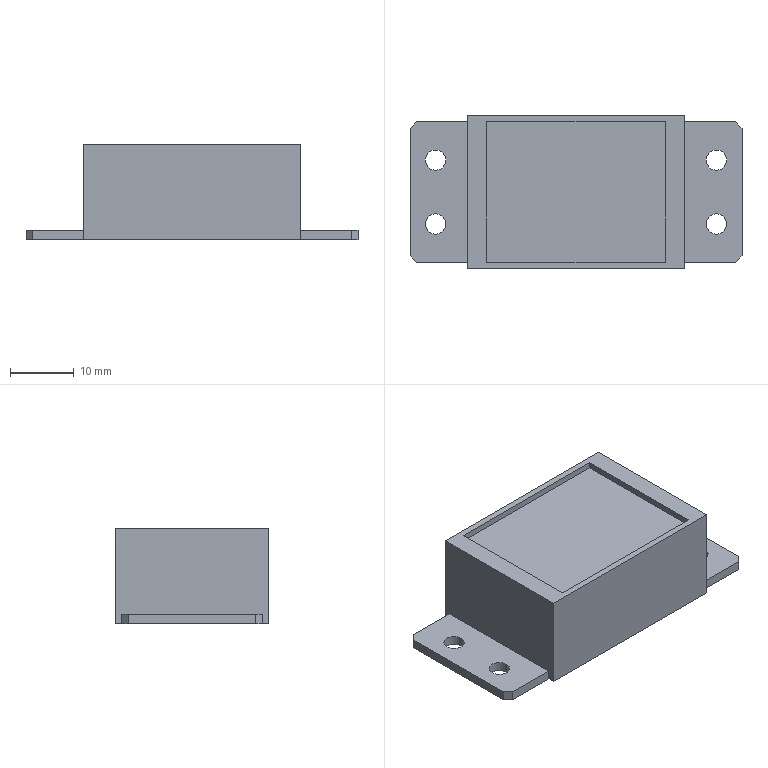Part | STEP file | V-light-BGS3-D20-R-W | 1 solid | 31 faces | box 52 x 24 x 15 mm | volume 12167 mm3 | plane 23 | cylinder 8 | commonest cylinder face diameters 3.2 x8
STEP:
#1=CARTESIAN_POINT('',(20.4,5.,0.));
#2=VERTEX_POINT('',#1);
#3=CARTESIAN_POINT('',(23.6,5.,0.));
#4=VERTEX_POINT('',#3);
#5=CARTESIAN_POINT('',(22.,5.,0.));
#6=DIRECTION('',(0.,0.,1.));
#7=DIRECTION('',(-1.,0.,0.));
#8=AXIS2_PLACEMENT_3D('',#5,#6,#7);
#9=CIRCLE('',#8,1.6);
#10=EDGE_CURVE('',#2,#4,#9,.T.);
#11=ORIENTED_EDGE('',*,*,#10,.F.);
#12=CARTESIAN_POINT('',(20.4,5.,1.5));
#13=VERTEX_POINT('',#12);
#14=CARTESIAN_POINT('',(20.4,5.,0.));
#15=DIRECTION('',(0.,0.,1.));
#16=VECTOR('',#15,1000.);
#17=LINE('',#14,#16);
#18=EDGE_CURVE('',#2,#13,#17,.T.);
#19=ORIENTED_EDGE('',*,*,#18,.T.);
#20=CARTESIAN_POINT('',(23.6,5.,1.5));
#21=VERTEX_POINT('',#20);
#22=CARTESIAN_POINT('',(22.,5.,1.5));
#23=DIRECTION('',(0.,0.,1.));
#24=DIRECTION('',(-1.,0.,0.));
#25=AXIS2_PLACEMENT_3D('',#22,#23,#24);
#26=CIRCLE('',#25,1.6);
#27=EDGE_CURVE('',#13,#21,#26,.T.);
#28=ORIENTED_EDGE('',*,*,#27,.T.);
#29=CARTESIAN_POINT('',(23.6,5.,0.));
#30=DIRECTION('',(0.,0.,1.));
#31=VECTOR('',#30,1000.);
#32=LINE('',#29,#31);
#33=EDGE_CURVE('',#4,#21,#32,.T.);
#34=ORIENTED_EDGE('',*,*,#33,.F.);
#35=EDGE_LOOP('',(#11,#19,#28,#34));
#36=FACE_OUTER_BOUND('',#35,.T.);
#37=CARTESIAN_POINT('',(22.,5.,0.));
#38=DIRECTION('',(0.,0.,1.));
#39=DIRECTION('',(1.,0.,0.));
#40=AXIS2_PLACEMENT_3D('',#37,#38,#39);
#41=CYLINDRICAL_SURFACE('',#40,1.6);
#42=ADVANCED_FACE('',(#36),#41,.F.);
#43=CARTESIAN_POINT('',(20.4,-5.,0.));
#44=VERTEX_POINT('',#43);
#45=CARTESIAN_POINT('',(23.6,-5.,0.));
#46=VERTEX_POINT('',#45);
#47=CARTESIAN_POINT('',(22.,-5.,0.));
#48=DIRECTION('',(0.,0.,1.));
#49=DIRECTION('',(1.,0.,0.));
#50=AXIS2_PLACEMENT_3D('',#47,#48,#49);
#51=CIRCLE('',#50,1.6);
#52=EDGE_CURVE('',#44,#46,#51,.T.);
#53=ORIENTED_EDGE('',*,*,#52,.F.);
#54=CARTESIAN_POINT('',(20.4,-5.,1.5));
#55=VERTEX_POINT('',#54);
#56=CARTESIAN_POINT('',(20.4,-5.,0.));
#57=DIRECTION('',(0.,0.,1.));
#58=VECTOR('',#57,1000.);
#59=LINE('',#56,#58);
#60=EDGE_CURVE('',#44,#55,#59,.T.);
#61=ORIENTED_EDGE('',*,*,#60,.T.);
#62=CARTESIAN_POINT('',(23.6,-5.,1.5));
#63=VERTEX_POINT('',#62);
#64=CARTESIAN_POINT('',(22.,-5.,1.5));
#65=DIRECTION('',(0.,0.,1.));
#66=DIRECTION('',(1.,0.,0.));
#67=AXIS2_PLACEMENT_3D('',#64,#65,#66);
#68=CIRCLE('',#67,1.6);
#69=EDGE_CURVE('',#55,#63,#68,.T.);
#70=ORIENTED_EDGE('',*,*,#69,.T.);
#71=CARTESIAN_POINT('',(23.6,-5.,0.));
#72=DIRECTION('',(0.,0.,1.));
#73=VECTOR('',#72,1000.);
#74=LINE('',#71,#73);
#75=EDGE_CURVE('',#46,#63,#74,.T.);
#76=ORIENTED_EDGE('',*,*,#75,.F.);
#77=EDGE_LOOP('',(#53,#61,#70,#76));
#78=FACE_OUTER_BOUND('',#77,.T.);
#79=CARTESIAN_POINT('',(22.,-5.,0.));
#80=DIRECTION('',(0.,0.,1.));
#81=DIRECTION('',(1.,0.,0.));
#82=AXIS2_PLACEMENT_3D('',#79,#80,#81);
#83=CYLINDRICAL_SURFACE('',#82,1.6);
#84=ADVANCED_FACE('',(#78),#83,.F.);
#85=CARTESIAN_POINT('',(-23.6,-5.,0.));
#86=VERTEX_POINT('',#85);
#87=CARTESIAN_POINT('',(-20.4,-5.,0.));
#88=VERTEX_POINT('',#87);
#89=CARTESIAN_POINT('',(-22.,-5.,0.));
#90=DIRECTION('',(0.,0.,1.));
#91=DIRECTION('',(-1.,0.,0.));
#92=AXIS2_PLACEMENT_3D('',#89,#90,#91);
#93=CIRCLE('',#92,1.6);
#94=EDGE_CURVE('',#86,#88,#93,.T.);
#95=ORIENTED_EDGE('',*,*,#94,.F.);
#96=CARTESIAN_POINT('',(-23.6,-5.,1.5));
#97=VERTEX_POINT('',#96);
#98=CARTESIAN_POINT('',(-23.6,-5.,0.));
#99=DIRECTION('',(0.,0.,1.));
#100=VECTOR('',#99,1000.);
#101=LINE('',#98,#100);
#102=EDGE_CURVE('',#86,#97,#101,.T.);
#103=ORIENTED_EDGE('',*,*,#102,.T.);
#104=CARTESIAN_POINT('',(-20.4,-5.,1.5));
#105=VERTEX_POINT('',#104);
#106=CARTESIAN_POINT('',(-22.,-5.,1.5));
#107=DIRECTION('',(0.,0.,1.));
#108=DIRECTION('',(-1.,0.,0.));
#109=AXIS2_PLACEMENT_3D('',#106,#107,#108);
#110=CIRCLE('',#109,1.6);
#111=EDGE_CURVE('',#97,#105,#110,.T.);
#112=ORIENTED_EDGE('',*,*,#111,.T.);
#113=CARTESIAN_POINT('',(-20.4,-5.,0.));
#114=DIRECTION('',(0.,0.,1.));
#115=VECTOR('',#114,1000.);
#116=LINE('',#113,#115);
#117=EDGE_CURVE('',#88,#105,#116,.T.);
#118=ORIENTED_EDGE('',*,*,#117,.F.);
#119=EDGE_LOOP('',(#95,#103,#112,#118));
#120=FACE_OUTER_BOUND('',#119,.T.);
#121=CARTESIAN_POINT('',(-22.,-5.,0.));
#122=DIRECTION('',(0.,0.,1.));
#123=DIRECTION('',(1.,0.,0.));
#124=AXIS2_PLACEMENT_3D('',#121,#122,#123);
#125=CYLINDRICAL_SURFACE('',#124,1.6);
#126=ADVANCED_FACE('',(#120),#125,.F.);
#127=CARTESIAN_POINT('',(-23.6,5.,0.));
#128=VERTEX_POINT('',#127);
#129=CARTESIAN_POINT('',(-20.4,5.,0.));
#130=VERTEX_POINT('',#129);
#131=CARTESIAN_POINT('',(-22.,5.,0.));
#132=DIRECTION('',(0.,0.,1.));
#133=DIRECTION('',(1.,0.,0.));
#134=AXIS2_PLACEMENT_3D('',#131,#132,#133);
#135=CIRCLE('',#134,1.6);
#136=EDGE_CURVE('',#128,#130,#135,.T.);
#137=ORIENTED_EDGE('',*,*,#136,.F.);
#138=CARTESIAN_POINT('',(-23.6,5.,1.5));
#139=VERTEX_POINT('',#138);
#140=CARTESIAN_POINT('',(-23.6,5.,0.));
#141=DIRECTION('',(0.,0.,1.));
#142=VECTOR('',#141,1000.);
#143=LINE('',#140,#142);
#144=EDGE_CURVE('',#128,#139,#143,.T.);
#145=ORIENTED_EDGE('',*,*,#144,.T.);
#146=CARTESIAN_POINT('',(-20.4,5.,1.5));
#147=VERTEX_POINT('',#146);
#148=CARTESIAN_POINT('',(-22.,5.,1.5));
#149=DIRECTION('',(0.,0.,1.));
#150=DIRECTION('',(1.,0.,0.));
#151=AXIS2_PLACEMENT_3D('',#148,#149,#150);
#152=CIRCLE('',#151,1.6);
#153=EDGE_CURVE('',#139,#147,#152,.T.);
#154=ORIENTED_EDGE('',*,*,#153,.T.);
#155=CARTESIAN_POINT('',(-20.4,5.,0.));
#156=DIRECTION('',(0.,0.,1.));
#157=VECTOR('',#156,1000.);
#158=LINE('',#155,#157);
#159=EDGE_CURVE('',#130,#147,#158,.T.);
#160=ORIENTED_EDGE('',*,*,#159,.F.);
#161=EDGE_LOOP('',(#137,#145,#154,#160));
#162=FACE_OUTER_BOUND('',#161,.T.);
#163=CARTESIAN_POINT('',(-22.,5.,0.));
#164=DIRECTION('',(0.,0.,1.));
#165=DIRECTION('',(1.,0.,0.));
#166=AXIS2_PLACEMENT_3D('',#163,#164,#165);
#167=CYLINDRICAL_SURFACE('',#166,1.6);
#168=ADVANCED_FACE('',(#162),#167,.F.);
#169=CARTESIAN_POINT('',(25.,-11.,1.5));
#170=VERTEX_POINT('',#169);
#171=CARTESIAN_POINT('',(17.,-11.,1.5));
#172=VERTEX_POINT('',#171);
#173=CARTESIAN_POINT('',(26.,-11.,1.5));
#174=DIRECTION('',(-1.,0.,0.));
#175=VECTOR('',#174,1000.);
#176=LINE('',#173,#175);
#177=EDGE_CURVE('',#170,#172,#176,.T.);
#178=ORIENTED_EDGE('',*,*,#177,.F.);
#179=CARTESIAN_POINT('',(26.,-10.,1.5));
#180=VERTEX_POINT('',#179);
#181=CARTESIAN_POINT('',(25.,-11.,1.5));
#182=DIRECTION('',(0.7071,0.7071,0.));
#183=VECTOR('',#182,1000.);
#184=LINE('',#181,#183);
#185=EDGE_CURVE('',#170,#180,#184,.T.);
#186=ORIENTED_EDGE('',*,*,#185,.T.);
#187=CARTESIAN_POINT('',(26.,10.,1.5));
#188=VERTEX_POINT('',#187);
#189=CARTESIAN_POINT('',(26.,12.,1.5));
#190=DIRECTION('',(0.,1.,0.));
#191=VECTOR('',#190,1000.);
#192=LINE('',#189,#191);
#193=EDGE_CURVE('',#180,#188,#192,.T.);
#194=ORIENTED_EDGE('',*,*,#193,.T.);
#195=CARTESIAN_POINT('',(25.,11.,1.5));
#196=VERTEX_POINT('',#195);
#197=CARTESIAN_POINT('',(37.,-1.,1.5));
#198=DIRECTION('',(-0.7071,0.7071,0.));
#199=VECTOR('',#198,1000.);
#200=LINE('',#197,#199);
#201=EDGE_CURVE('',#188,#196,#200,.T.);
#202=ORIENTED_EDGE('',*,*,#201,.T.);
#203=CARTESIAN_POINT('',(17.,11.,1.5));
#204=VERTEX_POINT('',#203);
#205=CARTESIAN_POINT('',(17.,11.,1.5));
#206=DIRECTION('',(1.,0.,0.));
#207=VECTOR('',#206,1000.);
#208=LINE('',#205,#207);
#209=EDGE_CURVE('',#204,#196,#208,.T.);
#210=ORIENTED_EDGE('',*,*,#209,.F.);
#211=CARTESIAN_POINT('',(17.,-12.,1.5));
#212=DIRECTION('',(0.,1.,0.));
#213=VECTOR('',#212,1000.);
#214=LINE('',#211,#213);
#215=EDGE_CURVE('',#172,#204,#214,.T.);
#216=ORIENTED_EDGE('',*,*,#215,.F.);
#217=EDGE_LOOP('',(#178,#186,#194,#202,#210,#216));
#218=FACE_OUTER_BOUND('',#217,.T.);
#219=CARTESIAN_POINT('',(22.,-5.,1.5));
#220=DIRECTION('',(0.,0.,1.));
#221=DIRECTION('',(1.,0.,0.));
#222=AXIS2_PLACEMENT_3D('',#219,#220,#221);
#223=CIRCLE('',#222,1.6);
#224=EDGE_CURVE('',#63,#55,#223,.T.);
#225=ORIENTED_EDGE('',*,*,#224,.F.);
#226=ORIENTED_EDGE('',*,*,#69,.F.);
#227=EDGE_LOOP('',(#225,#226));
#228=FACE_BOUND('',#227,.T.);
#229=CARTESIAN_POINT('',(22.,5.,1.5));
#230=DIRECTION('',(0.,0.,1.));
#231=DIRECTION('',(-1.,0.,0.));
#232=AXIS2_PLACEMENT_3D('',#229,#230,#231);
#233=CIRCLE('',#232,1.6);
#234=EDGE_CURVE('',#21,#13,#233,.T.);
#235=ORIENTED_EDGE('',*,*,#234,.F.);
#236=ORIENTED_EDGE('',*,*,#27,.F.);
#237=EDGE_LOOP('',(#235,#236));
#238=FACE_BOUND('',#237,.T.);
#239=CARTESIAN_POINT('',(26.,-12.,1.5));
#240=DIRECTION('',(0.,0.,1.));
#241=DIRECTION('',(1.,0.,0.));
#242=AXIS2_PLACEMENT_3D('',#239,#240,#241);
#243=PLANE('',#242);
#244=ADVANCED_FACE('',(#218,#228,#238),#243,.T.);
#245=ORIENTED_EDGE('',*,*,#193,.F.);
#246=CARTESIAN_POINT('',(26.,-10.,0.));
#247=VERTEX_POINT('',#246);
#248=CARTESIAN_POINT('',(26.,-10.,1.5));
#249=DIRECTION('',(0.,0.,-1.));
#250=VECTOR('',#249,1000.);
#251=LINE('',#248,#250);
#252=EDGE_CURVE('',#180,#247,#251,.T.);
#253=ORIENTED_EDGE('',*,*,#252,.T.);
#254=CARTESIAN_POINT('',(26.,10.,0.));
#255=VERTEX_POINT('',#254);
#256=CARTESIAN_POINT('',(26.,12.,0.));
#257=DIRECTION('',(0.,1.,0.));
#258=VECTOR('',#257,1000.);
#259=LINE('',#256,#258);
#260=EDGE_CURVE('',#247,#255,#259,.T.);
#261=ORIENTED_EDGE('',*,*,#260,.T.);
#262=CARTESIAN_POINT('',(26.,10.,1.5));
#263=DIRECTION('',(0.,0.,1.));
#264=VECTOR('',#263,1000.);
#265=LINE('',#262,#264);
#266=EDGE_CURVE('',#255,#188,#265,.T.);
#267=ORIENTED_EDGE('',*,*,#266,.T.);
#268=EDGE_LOOP('',(#245,#253,#261,#267));
#269=FACE_OUTER_BOUND('',#268,.T.);
#270=CARTESIAN_POINT('',(26.,12.,1.5));
#271=DIRECTION('',(-1.,0.,0.));
#272=DIRECTION('',(0.,-1.,0.));
#273=AXIS2_PLACEMENT_3D('',#270,#271,#272);
#274=PLANE('',#273);
#275=ADVANCED_FACE('',(#269),#274,.F.);
#276=CARTESIAN_POINT('',(17.,12.,0.));
#277=VERTEX_POINT('',#276);
#278=CARTESIAN_POINT('',(-17.,12.,0.));
#279=VERTEX_POINT('',#278);
#280=CARTESIAN_POINT('',(-26.,12.,0.));
#281=DIRECTION('',(-1.,0.,0.));
#282=VECTOR('',#281,1000.);
#283=LINE('',#280,#282);
#284=EDGE_CURVE('',#277,#279,#283,.T.);
#285=ORIENTED_EDGE('',*,*,#284,.T.);
#286=CARTESIAN_POINT('',(-17.,12.,15.));
#287=VERTEX_POINT('',#286);
#288=CARTESIAN_POINT('',(-17.,12.,15.));
#289=DIRECTION('',(0.,0.,-1.));
#290=VECTOR('',#289,1000.);
#291=LINE('',#288,#290);
#292=EDGE_CURVE('',#287,#279,#291,.T.);
#293=ORIENTED_EDGE('',*,*,#292,.F.);
#294=CARTESIAN_POINT('',(17.,12.,15.));
#295=VERTEX_POINT('',#294);
#296=CARTESIAN_POINT('',(-17.,12.,15.));
#297=DIRECTION('',(-1.,0.,0.));
#298=VECTOR('',#297,1000.);
#299=LINE('',#296,#298);
#300=EDGE_CURVE('',#295,#287,#299,.T.);
#301=ORIENTED_EDGE('',*,*,#300,.F.);
#302=CARTESIAN_POINT('',(17.,12.,15.));
#303=DIRECTION('',(0.,0.,-1.));
#304=VECTOR('',#303,1000.);
#305=LINE('',#302,#304);
#306=EDGE_CURVE('',#295,#277,#305,.T.);
#307=ORIENTED_EDGE('',*,*,#306,.T.);
#308=EDGE_LOOP('',(#285,#293,#301,#307));
#309=FACE_OUTER_BOUND('',#308,.T.);
#310=CARTESIAN_POINT('',(-26.,12.,1.5));
#311=DIRECTION('',(0.,-1.,0.));
#312=DIRECTION('',(0.,0.,-1.));
#313=AXIS2_PLACEMENT_3D('',#310,#311,#312);
#314=PLANE('',#313);
#315=ADVANCED_FACE('',(#309),#314,.F.);
#316=CARTESIAN_POINT('',(-26.,10.,0.));
#317=VERTEX_POINT('',#316);
#318=CARTESIAN_POINT('',(-26.,-10.,0.));
#319=VERTEX_POINT('',#318);
#320=CARTESIAN_POINT('',(-26.,12.,0.));
#321=DIRECTION('',(0.,-1.,0.));
#322=VECTOR('',#321,1000.);
#323=LINE('',#320,#322);
#324=EDGE_CURVE('',#317,#319,#323,.T.);
#325=ORIENTED_EDGE('',*,*,#324,.T.);
#326=CARTESIAN_POINT('',(-26.,-10.,1.5));
#327=VERTEX_POINT('',#326);
#328=CARTESIAN_POINT('',(-26.,-10.,1.5));
#329=DIRECTION('',(0.,0.,1.));
#330=VECTOR('',#329,1000.);
#331=LINE('',#328,#330);
#332=EDGE_CURVE('',#319,#327,#331,.T.);
#333=ORIENTED_EDGE('',*,*,#332,.T.);
#334=CARTESIAN_POINT('',(-26.,10.,1.5));
#335=VERTEX_POINT('',#334);
#336=CARTESIAN_POINT('',(-26.,12.,1.5));
#337=DIRECTION('',(0.,-1.,0.));
#338=VECTOR('',#337,1000.);
#339=LINE('',#336,#338);
#340=EDGE_CURVE('',#335,#327,#339,.T.);
#341=ORIENTED_EDGE('',*,*,#340,.F.);
#342=CARTESIAN_POINT('',(-26.,10.,1.5));
#343=DIRECTION('',(0.,0.,-1.));
#344=VECTOR('',#343,1000.);
#345=LINE('',#342,#344);
#346=EDGE_CURVE('',#335,#317,#345,.T.);
#347=ORIENTED_EDGE('',*,*,#346,.T.);
#348=EDGE_LOOP('',(#325,#333,#341,#347));
#349=FACE_OUTER_BOUND('',#348,.T.);
#350=CARTESIAN_POINT('',(-26.,12.,1.5));
#351=DIRECTION('',(1.,0.,0.));
#352=DIRECTION('',(0.,1.,0.));
#353=AXIS2_PLACEMENT_3D('',#350,#351,#352);
#354=PLANE('',#353);
#355=ADVANCED_FACE('',(#349),#354,.F.);
#356=CARTESIAN_POINT('',(-17.,-12.,15.));
#357=VERTEX_POINT('',#356);
#358=CARTESIAN_POINT('',(-17.,-12.,0.));
#359=VERTEX_POINT('',#358);
#360=CARTESIAN_POINT('',(-17.,-12.,15.));
#361=DIRECTION('',(0.,0.,-1.));
#362=VECTOR('',#361,1000.);
#363=LINE('',#360,#362);
#364=EDGE_CURVE('',#357,#359,#363,.T.);
#365=ORIENTED_EDGE('',*,*,#364,.T.);
#366=CARTESIAN_POINT('',(17.,-12.,0.));
#367=VERTEX_POINT('',#366);
#368=CARTESIAN_POINT('',(-26.,-12.,0.));
#369=DIRECTION('',(1.,0.,0.));
#370=VECTOR('',#369,1000.);
#371=LINE('',#368,#370);
#372=EDGE_CURVE('',#359,#367,#371,.T.);
#373=ORIENTED_EDGE('',*,*,#372,.T.);
#374=CARTESIAN_POINT('',(17.,-12.,15.));
#375=VERTEX_POINT('',#374);
#376=CARTESIAN_POINT('',(17.,-12.,15.));
#377=DIRECTION('',(0.,0.,-1.));
#378=VECTOR('',#377,1000.);
#379=LINE('',#376,#378);
#380=EDGE_CURVE('',#375,#367,#379,.T.);
#381=ORIENTED_EDGE('',*,*,#380,.F.);
#382=CARTESIAN_POINT('',(-17.,-12.,15.));
#383=DIRECTION('',(1.,0.,0.));
#384=VECTOR('',#383,1000.);
#385=LINE('',#382,#384);
#386=EDGE_CURVE('',#357,#375,#385,.T.);
#387=ORIENTED_EDGE('',*,*,#386,.F.);
#388=EDGE_LOOP('',(#365,#373,#381,#387));
#389=FACE_OUTER_BOUND('',#388,.T.);
#390=CARTESIAN_POINT('',(-26.,-12.,1.5));
#391=DIRECTION('',(0.,1.,0.));
#392=DIRECTION('',(0.,0.,1.));
#393=AXIS2_PLACEMENT_3D('',#390,#391,#392);
#394=PLANE('',#393);
#395=ADVANCED_FACE('',(#389),#394,.F.);
#396=ORIENTED_EDGE('',*,*,#340,.T.);
#397=CARTESIAN_POINT('',(-25.,-11.,1.5));
#398=VERTEX_POINT('',#397);
#399=CARTESIAN_POINT('',(1.,-37.,1.5));
#400=DIRECTION('',(0.7071,-0.7071,0.));
#401=VECTOR('',#400,1000.);
#402=LINE('',#399,#401);
#403=EDGE_CURVE('',#327,#398,#402,.T.);
#404=ORIENTED_EDGE('',*,*,#403,.T.);
#405=CARTESIAN_POINT('',(-17.,-11.,1.5));
#406=VERTEX_POINT('',#405);
#407=CARTESIAN_POINT('',(-26.,-11.,1.5));
#408=DIRECTION('',(-1.,0.,0.));
#409=VECTOR('',#408,1000.);
#410=LINE('',#407,#409);
#411=EDGE_CURVE('',#406,#398,#410,.T.);
#412=ORIENTED_EDGE('',*,*,#411,.F.);
#413=CARTESIAN_POINT('',(-17.,11.,1.5));
#414=VERTEX_POINT('',#413);
#415=CARTESIAN_POINT('',(-17.,-12.,1.5));
#416=DIRECTION('',(0.,-1.,0.));
#417=VECTOR('',#416,1000.);
#418=LINE('',#415,#417);
#419=EDGE_CURVE('',#414,#406,#418,.T.);
#420=ORIENTED_EDGE('',*,*,#419,.F.);
#421=CARTESIAN_POINT('',(-25.,11.,1.5));
#422=VERTEX_POINT('',#421);
#423=CARTESIAN_POINT('',(-17.,11.,1.5));
#424=DIRECTION('',(1.,0.,0.));
#425=VECTOR('',#424,1000.);
#426=LINE('',#423,#425);
#427=EDGE_CURVE('',#422,#414,#426,.T.);
#428=ORIENTED_EDGE('',*,*,#427,.F.);
#429=CARTESIAN_POINT('',(-11.,25.,1.5));
#430=DIRECTION('',(-0.7071,-0.7071,0.));
#431=VECTOR('',#430,1000.);
#432=LINE('',#429,#431);
#433=EDGE_CURVE('',#422,#335,#432,.T.);
#434=ORIENTED_EDGE('',*,*,#433,.T.);
#435=EDGE_LOOP('',(#396,#404,#412,#420,#428,#434));
#436=FACE_OUTER_BOUND('',#435,.T.);
#437=CARTESIAN_POINT('',(-22.,-5.,1.5));
#438=DIRECTION('',(0.,0.,1.));
#439=DIRECTION('',(-1.,0.,0.));
#440=AXIS2_PLACEMENT_3D('',#437,#438,#439);
#441=CIRCLE('',#440,1.6);
#442=EDGE_CURVE('',#105,#97,#441,.T.);
#443=ORIENTED_EDGE('',*,*,#442,.F.);
#444=ORIENTED_EDGE('',*,*,#111,.F.);
#445=EDGE_LOOP('',(#443,#444));
#446=FACE_BOUND('',#445,.T.);
#447=CARTESIAN_POINT('',(-22.,5.,1.5));
#448=DIRECTION('',(0.,0.,1.));
#449=DIRECTION('',(1.,0.,0.));
#450=AXIS2_PLACEMENT_3D('',#447,#448,#449);
#451=CIRCLE('',#450,1.6);
#452=EDGE_CURVE('',#147,#139,#451,.T.);
#453=ORIENTED_EDGE('',*,*,#452,.F.);
#454=ORIENTED_EDGE('',*,*,#153,.F.);
#455=EDGE_LOOP('',(#453,#454));
#456=FACE_BOUND('',#455,.T.);
#457=CARTESIAN_POINT('',(26.,-12.,1.5));
#458=DIRECTION('',(0.,0.,1.));
#459=DIRECTION('',(1.,0.,0.));
#460=AXIS2_PLACEMENT_3D('',#457,#458,#459);
#461=PLANE('',#460);
#462=ADVANCED_FACE('',(#436,#446,#456),#461,.T.);
#463=CARTESIAN_POINT('',(22.,5.,0.));
#464=DIRECTION('',(0.,0.,1.));
#465=DIRECTION('',(-1.,0.,0.));
#466=AXIS2_PLACEMENT_3D('',#463,#464,#465);
#467=CIRCLE('',#466,1.6);
#468=EDGE_CURVE('',#4,#2,#467,.T.);
#469=ORIENTED_EDGE('',*,*,#468,.T.);
#470=ORIENTED_EDGE('',*,*,#10,.T.);
#471=EDGE_LOOP('',(#469,#470));
#472=FACE_BOUND('',#471,.T.);
#473=CARTESIAN_POINT('',(22.,-5.,0.));
#474=DIRECTION('',(0.,0.,1.));
#475=DIRECTION('',(1.,0.,0.));
#476=AXIS2_PLACEMENT_3D('',#473,#474,#475);
#477=CIRCLE('',#476,1.6);
#478=EDGE_CURVE('',#46,#44,#477,.T.);
#479=ORIENTED_EDGE('',*,*,#478,.T.);
#480=ORIENTED_EDGE('',*,*,#52,.T.);
#481=EDGE_LOOP('',(#479,#480));
#482=FACE_BOUND('',#481,.T.);
#483=CARTESIAN_POINT('',(-22.,-5.,0.));
#484=DIRECTION('',(0.,0.,1.));
#485=DIRECTION('',(-1.,0.,0.));
#486=AXIS2_PLACEMENT_3D('',#483,#484,#485);
#487=CIRCLE('',#486,1.6);
#488=EDGE_CURVE('',#88,#86,#487,.T.);
#489=ORIENTED_EDGE('',*,*,#488,.T.);
#490=ORIENTED_EDGE('',*,*,#94,.T.);
#491=EDGE_LOOP('',(#489,#490));
#492=FACE_BOUND('',#491,.T.);
#493=CARTESIAN_POINT('',(-22.,5.,0.));
#494=DIRECTION('',(0.,0.,1.));
#495=DIRECTION('',(1.,0.,0.));
#496=AXIS2_PLACEMENT_3D('',#493,#494,#495);
#497=CIRCLE('',#496,1.6);
#498=EDGE_CURVE('',#130,#128,#497,.T.);
#499=ORIENTED_EDGE('',*,*,#498,.T.);
#500=ORIENTED_EDGE('',*,*,#136,.T.);
#501=EDGE_LOOP('',(#499,#500));
#502=FACE_BOUND('',#501,.T.);
#503=CARTESIAN_POINT('',(-17.,-11.,0.));
#504=VERTEX_POINT('',#503);
#505=CARTESIAN_POINT('',(-25.,-11.,0.));
#506=VERTEX_POINT('',#505);
#507=CARTESIAN_POINT('',(26.,-11.,0.));
#508=DIRECTION('',(-1.,0.,0.));
#509=VECTOR('',#508,1000.);
#510=LINE('',#507,#509);
#511=EDGE_CURVE('',#504,#506,#510,.T.);
#512=ORIENTED_EDGE('',*,*,#511,.T.);
#513=CARTESIAN_POINT('',(-26.,-10.,0.));
#514=DIRECTION('',(-0.7071,0.7071,0.));
#515=VECTOR('',#514,1000.);
#516=LINE('',#513,#515);
#517=EDGE_CURVE('',#506,#319,#516,.T.);
#518=ORIENTED_EDGE('',*,*,#517,.T.);
#519=ORIENTED_EDGE('',*,*,#324,.F.);
#520=CARTESIAN_POINT('',(-25.,11.,0.));
#521=VERTEX_POINT('',#520);
#522=CARTESIAN_POINT('',(-26.,10.,0.));
#523=DIRECTION('',(0.7071,0.7071,0.));
#524=VECTOR('',#523,1000.);
#525=LINE('',#522,#524);
#526=EDGE_CURVE('',#317,#521,#525,.T.);
#527=ORIENTED_EDGE('',*,*,#526,.T.);
#528=CARTESIAN_POINT('',(-17.,11.,0.));
#529=VERTEX_POINT('',#528);
#530=CARTESIAN_POINT('',(26.,11.,0.));
#531=DIRECTION('',(1.,0.,0.));
#532=VECTOR('',#531,1000.);
#533=LINE('',#530,#532);
#534=EDGE_CURVE('',#521,#529,#533,.T.);
#535=ORIENTED_EDGE('',*,*,#534,.T.);
#536=CARTESIAN_POINT('',(-17.,-12.,0.));
#537=DIRECTION('',(0.,1.,0.));
#538=VECTOR('',#537,1000.);
#539=LINE('',#536,#538);
#540=EDGE_CURVE('',#529,#279,#539,.T.);
#541=ORIENTED_EDGE('',*,*,#540,.T.);
#542=ORIENTED_EDGE('',*,*,#284,.F.);
#543=CARTESIAN_POINT('',(17.,11.,0.));
#544=VERTEX_POINT('',#543);
#545=CARTESIAN_POINT('',(17.,-12.,0.));
#546=DIRECTION('',(0.,-1.,0.));
#547=VECTOR('',#546,1000.);
#548=LINE('',#545,#547);
#549=EDGE_CURVE('',#277,#544,#548,.T.);
#550=ORIENTED_EDGE('',*,*,#549,.T.);
#551=CARTESIAN_POINT('',(25.,11.,0.));
#552=VERTEX_POINT('',#551);
#553=CARTESIAN_POINT('',(26.,11.,0.));
#554=DIRECTION('',(1.,0.,0.));
#555=VECTOR('',#554,1000.);
#556=LINE('',#553,#555);
#557=EDGE_CURVE('',#544,#552,#556,.T.);
#558=ORIENTED_EDGE('',*,*,#557,.T.);
#559=CARTESIAN_POINT('',(26.,10.,0.));
#560=DIRECTION('',(0.7071,-0.7071,0.));
#561=VECTOR('',#560,1000.);
#562=LINE('',#559,#561);
#563=EDGE_CURVE('',#552,#255,#562,.T.);
#564=ORIENTED_EDGE('',*,*,#563,.T.);
#565=ORIENTED_EDGE('',*,*,#260,.F.);
#566=CARTESIAN_POINT('',(25.,-11.,0.));
#567=VERTEX_POINT('',#566);
#568=CARTESIAN_POINT('',(25.,-11.,0.));
#569=DIRECTION('',(-0.7071,-0.7071,0.));
#570=VECTOR('',#569,1000.);
#571=LINE('',#568,#570);
#572=EDGE_CURVE('',#247,#567,#571,.T.);
#573=ORIENTED_EDGE('',*,*,#572,.T.);
#574=CARTESIAN_POINT('',(17.,-11.,0.));
#575=VERTEX_POINT('',#574);
#576=CARTESIAN_POINT('',(26.,-11.,0.));
#577=DIRECTION('',(-1.,0.,0.));
#578=VECTOR('',#577,1000.);
#579=LINE('',#576,#578);
#580=EDGE_CURVE('',#567,#575,#579,.T.);
#581=ORIENTED_EDGE('',*,*,#580,.T.);
#582=CARTESIAN_POINT('',(17.,-12.,0.));
#583=DIRECTION('',(0.,-1.,0.));
#584=VECTOR('',#583,1000.);
#585=LINE('',#582,#584);
#586=EDGE_CURVE('',#575,#367,#585,.T.);
#587=ORIENTED_EDGE('',*,*,#586,.T.);
#588=ORIENTED_EDGE('',*,*,#372,.F.);
#589=CARTESIAN_POINT('',(-17.,-12.,0.));
#590=DIRECTION('',(0.,1.,0.));
#591=VECTOR('',#590,1000.);
#592=LINE('',#589,#591);
#593=EDGE_CURVE('',#359,#504,#592,.T.);
#594=ORIENTED_EDGE('',*,*,#593,.T.);
#595=EDGE_LOOP('',(#512,#518,#519,#527,#535,#541,#542,#550,#558,#564,#565,#573,#581,#587,#588,#594));
#596=FACE_OUTER_BOUND('',#595,.T.);
#597=CARTESIAN_POINT('',(26.,-12.,0.));
#598=DIRECTION('',(0.,0.,1.));
#599=DIRECTION('',(1.,0.,0.));
#600=AXIS2_PLACEMENT_3D('',#597,#598,#599);
#601=PLANE('',#600);
#602=ADVANCED_FACE('',(#472,#482,#492,#502,#596),#601,.F.);
#603=ORIENTED_EDGE('',*,*,#144,.F.);
#604=ORIENTED_EDGE('',*,*,#498,.F.);
#605=ORIENTED_EDGE('',*,*,#159,.T.);
#606=ORIENTED_EDGE('',*,*,#452,.T.);
#607=EDGE_LOOP('',(#603,#604,#605,#606));
#608=FACE_OUTER_BOUND('',#607,.T.);
#609=CARTESIAN_POINT('',(-22.,5.,0.));
#610=DIRECTION('',(0.,0.,1.));
#611=DIRECTION('',(1.,0.,0.));
#612=AXIS2_PLACEMENT_3D('',#609,#610,#611);
#613=CYLINDRICAL_SURFACE('',#612,1.6);
#614=ADVANCED_FACE('',(#608),#613,.F.);
#615=ORIENTED_EDGE('',*,*,#102,.F.);
#616=ORIENTED_EDGE('',*,*,#488,.F.);
#617=ORIENTED_EDGE('',*,*,#117,.T.);
#618=ORIENTED_EDGE('',*,*,#442,.T.);
#619=EDGE_LOOP('',(#615,#616,#617,#618));
#620=FACE_OUTER_BOUND('',#619,.T.);
#621=CARTESIAN_POINT('',(-22.,-5.,0.));
#622=DIRECTION('',(0.,0.,1.));
#623=DIRECTION('',(1.,0.,0.));
#624=AXIS2_PLACEMENT_3D('',#621,#622,#623);
#625=CYLINDRICAL_SURFACE('',#624,1.6);
#626=ADVANCED_FACE('',(#620),#625,.F.);
#627=ORIENTED_EDGE('',*,*,#60,.F.);
#628=ORIENTED_EDGE('',*,*,#478,.F.);
#629=ORIENTED_EDGE('',*,*,#75,.T.);
#630=ORIENTED_EDGE('',*,*,#224,.T.);
#631=EDGE_LOOP('',(#627,#628,#629,#630));
#632=FACE_OUTER_BOUND('',#631,.T.);
#633=CARTESIAN_POINT('',(22.,-5.,0.));
#634=DIRECTION('',(0.,0.,1.));
#635=DIRECTION('',(1.,0.,0.));
#636=AXIS2_PLACEMENT_3D('',#633,#634,#635);
#637=CYLINDRICAL_SURFACE('',#636,1.6);
#638=ADVANCED_FACE('',(#632),#637,.F.);
#639=ORIENTED_EDGE('',*,*,#18,.F.);
#640=ORIENTED_EDGE('',*,*,#468,.F.);
#641=ORIENTED_EDGE('',*,*,#33,.T.);
#642=ORIENTED_EDGE('',*,*,#234,.T.);
#643=EDGE_LOOP('',(#639,#640,#641,#642));
#644=FACE_OUTER_BOUND('',#643,.T.);
#645=CARTESIAN_POINT('',(22.,5.,0.));
#646=DIRECTION('',(0.,0.,1.));
#647=DIRECTION('',(1.,0.,0.));
#648=AXIS2_PLACEMENT_3D('',#645,#646,#647);
#649=CYLINDRICAL_SURFACE('',#648,1.6);
#650=ADVANCED_FACE('',(#644),#649,.F.);
#651=ORIENTED_EDGE('',*,*,#380,.T.);
#652=ORIENTED_EDGE('',*,*,#586,.F.);
#653=CARTESIAN_POINT('',(17.,-11.,-3.5));
#654=DIRECTION('',(0.,0.,1.));
#655=VECTOR('',#654,1000.);
#656=LINE('',#653,#655);
#657=EDGE_CURVE('',#575,#172,#656,.T.);
#658=ORIENTED_EDGE('',*,*,#657,.T.);
#659=ORIENTED_EDGE('',*,*,#215,.T.);
#660=CARTESIAN_POINT('',(17.,11.,-3.5));
#661=DIRECTION('',(0.,0.,1.));
#662=VECTOR('',#661,1000.);
#663=LINE('',#660,#662);
#664=EDGE_CURVE('',#544,#204,#663,.T.);
#665=ORIENTED_EDGE('',*,*,#664,.F.);
#666=ORIENTED_EDGE('',*,*,#549,.F.);
#667=ORIENTED_EDGE('',*,*,#306,.F.);
#668=CARTESIAN_POINT('',(17.,-12.,15.));
#669=DIRECTION('',(0.,1.,0.));
#670=VECTOR('',#669,1000.);
#671=LINE('',#668,#670);
#672=EDGE_CURVE('',#375,#295,#671,.T.);
#673=ORIENTED_EDGE('',*,*,#672,.F.);
#674=EDGE_LOOP('',(#651,#652,#658,#659,#665,#666,#667,#673));
#675=FACE_OUTER_BOUND('',#674,.T.);
#676=CARTESIAN_POINT('',(17.,-12.,15.));
#677=DIRECTION('',(-1.,0.,0.));
#678=DIRECTION('',(0.,0.,1.));
#679=AXIS2_PLACEMENT_3D('',#676,#677,#678);
#680=PLANE('',#679);
#681=ADVANCED_FACE('',(#675),#680,.F.);
#682=ORIENTED_EDGE('',*,*,#292,.T.);
#683=ORIENTED_EDGE('',*,*,#540,.F.);
#684=CARTESIAN_POINT('',(-17.,11.,-3.5));
#685=DIRECTION('',(0.,0.,1.));
#686=VECTOR('',#685,1000.);
#687=LINE('',#684,#686);
#688=EDGE_CURVE('',#529,#414,#687,.T.);
#689=ORIENTED_EDGE('',*,*,#688,.T.);
#690=ORIENTED_EDGE('',*,*,#419,.T.);
#691=CARTESIAN_POINT('',(-17.,-11.,-3.5));
#692=DIRECTION('',(0.,0.,1.));
#693=VECTOR('',#692,1000.);
#694=LINE('',#691,#693);
#695=EDGE_CURVE('',#504,#406,#694,.T.);
#696=ORIENTED_EDGE('',*,*,#695,.F.);
#697=ORIENTED_EDGE('',*,*,#593,.F.);
#698=ORIENTED_EDGE('',*,*,#364,.F.);
#699=CARTESIAN_POINT('',(-17.,-12.,15.));
#700=DIRECTION('',(0.,-1.,0.));
#701=VECTOR('',#700,1000.);
#702=LINE('',#699,#701);
#703=EDGE_CURVE('',#287,#357,#702,.T.);
#704=ORIENTED_EDGE('',*,*,#703,.F.);
#705=EDGE_LOOP('',(#682,#683,#689,#690,#696,#697,#698,#704));
#706=FACE_OUTER_BOUND('',#705,.T.);
#707=CARTESIAN_POINT('',(-17.,-12.,15.));
#708=DIRECTION('',(1.,0.,0.));
#709=DIRECTION('',(0.,0.,-1.));
#710=AXIS2_PLACEMENT_3D('',#707,#708,#709);
#711=PLANE('',#710);
#712=ADVANCED_FACE('',(#706),#711,.F.);
#713=CARTESIAN_POINT('',(14.,11.,15.));
#714=VERTEX_POINT('',#713);
#715=CARTESIAN_POINT('',(-14.,11.,15.));
#716=VERTEX_POINT('',#715);
#717=CARTESIAN_POINT('',(-14.,11.,15.));
#718=DIRECTION('',(-1.,0.,0.));
#719=VECTOR('',#718,1000.);
#720=LINE('',#717,#719);
#721=EDGE_CURVE('',#714,#716,#720,.T.);
#722=ORIENTED_EDGE('',*,*,#721,.F.);
#723=CARTESIAN_POINT('',(14.,-11.,15.));
#724=VERTEX_POINT('',#723);
#725=CARTESIAN_POINT('',(14.,11.,15.));
#726=DIRECTION('',(0.,1.,0.));
#727=VECTOR('',#726,1000.);
#728=LINE('',#725,#727);
#729=EDGE_CURVE('',#724,#714,#728,.T.);
#730=ORIENTED_EDGE('',*,*,#729,.F.);
#731=CARTESIAN_POINT('',(-14.,-11.,15.));
#732=VERTEX_POINT('',#731);
#733=CARTESIAN_POINT('',(-14.,-11.,15.));
#734=DIRECTION('',(1.,0.,0.));
#735=VECTOR('',#734,1000.);
#736=LINE('',#733,#735);
#737=EDGE_CURVE('',#732,#724,#736,.T.);
#738=ORIENTED_EDGE('',*,*,#737,.F.);
#739=CARTESIAN_POINT('',(-14.,11.,15.));
#740=DIRECTION('',(0.,-1.,0.));
#741=VECTOR('',#740,1000.);
#742=LINE('',#739,#741);
#743=EDGE_CURVE('',#716,#732,#742,.T.);
#744=ORIENTED_EDGE('',*,*,#743,.F.);
#745=EDGE_LOOP('',(#722,#730,#738,#744));
#746=FACE_BOUND('',#745,.T.);
#747=ORIENTED_EDGE('',*,*,#672,.T.);
#748=ORIENTED_EDGE('',*,*,#300,.T.);
#749=ORIENTED_EDGE('',*,*,#703,.T.);
#750=ORIENTED_EDGE('',*,*,#386,.T.);
#751=EDGE_LOOP('',(#747,#748,#749,#750));
#752=FACE_OUTER_BOUND('',#751,.T.);
#753=CARTESIAN_POINT('',(17.,12.,15.));
#754=DIRECTION('',(0.,0.,-1.));
#755=DIRECTION('',(-1.,0.,0.));
#756=AXIS2_PLACEMENT_3D('',#753,#754,#755);
#757=PLANE('',#756);
#758=ADVANCED_FACE('',(#746,#752),#757,.F.);
#759=ORIENTED_EDGE('',*,*,#729,.T.);
#760=CARTESIAN_POINT('',(14.,11.,14.));
#761=VERTEX_POINT('',#760);
#762=CARTESIAN_POINT('',(14.,11.,14.));
#763=DIRECTION('',(0.,0.,1.));
#764=VECTOR('',#763,1000.);
#765=LINE('',#762,#764);
#766=EDGE_CURVE('',#761,#714,#765,.T.);
#767=ORIENTED_EDGE('',*,*,#766,.F.);
#768=CARTESIAN_POINT('',(14.,-11.,14.));
#769=VERTEX_POINT('',#768);
#770=CARTESIAN_POINT('',(14.,11.,14.));
#771=DIRECTION('',(0.,1.,0.));
#772=VECTOR('',#771,1000.);
#773=LINE('',#770,#772);
#774=EDGE_CURVE('',#769,#761,#773,.T.);
#775=ORIENTED_EDGE('',*,*,#774,.F.);
#776=CARTESIAN_POINT('',(14.,-11.,14.));
#777=DIRECTION('',(0.,0.,1.));
#778=VECTOR('',#777,1000.);
#779=LINE('',#776,#778);
#780=EDGE_CURVE('',#769,#724,#779,.T.);
#781=ORIENTED_EDGE('',*,*,#780,.T.);
#782=EDGE_LOOP('',(#759,#767,#775,#781));
#783=FACE_OUTER_BOUND('',#782,.T.);
#784=CARTESIAN_POINT('',(14.,11.,14.));
#785=DIRECTION('',(1.,0.,0.));
#786=DIRECTION('',(0.,1.,0.));
#787=AXIS2_PLACEMENT_3D('',#784,#785,#786);
#788=PLANE('',#787);
#789=ADVANCED_FACE('',(#783),#788,.F.);
#790=ORIENTED_EDGE('',*,*,#737,.T.);
#791=ORIENTED_EDGE('',*,*,#780,.F.);
#792=CARTESIAN_POINT('',(-14.,-11.,14.));
#793=VERTEX_POINT('',#792);
#794=CARTESIAN_POINT('',(-14.,-11.,14.));
#795=DIRECTION('',(1.,0.,0.));
#796=VECTOR('',#795,1000.);
#797=LINE('',#794,#796);
#798=EDGE_CURVE('',#793,#769,#797,.T.);
#799=ORIENTED_EDGE('',*,*,#798,.F.);
#800=CARTESIAN_POINT('',(-14.,-11.,14.));
#801=DIRECTION('',(0.,0.,1.));
#802=VECTOR('',#801,1000.);
#803=LINE('',#800,#802);
#804=EDGE_CURVE('',#793,#732,#803,.T.);
#805=ORIENTED_EDGE('',*,*,#804,.T.);
#806=EDGE_LOOP('',(#790,#791,#799,#805));
#807=FACE_OUTER_BOUND('',#806,.T.);
#808=CARTESIAN_POINT('',(-14.,-11.,14.));
#809=DIRECTION('',(0.,-1.,0.));
#810=DIRECTION('',(0.,0.,-1.));
#811=AXIS2_PLACEMENT_3D('',#808,#809,#810);
#812=PLANE('',#811);
#813=ADVANCED_FACE('',(#807),#812,.F.);
#814=ORIENTED_EDGE('',*,*,#743,.T.);
#815=ORIENTED_EDGE('',*,*,#804,.F.);
#816=CARTESIAN_POINT('',(-14.,11.,14.));
#817=VERTEX_POINT('',#816);
#818=CARTESIAN_POINT('',(-14.,11.,14.));
#819=DIRECTION('',(0.,-1.,0.));
#820=VECTOR('',#819,1000.);
#821=LINE('',#818,#820);
#822=EDGE_CURVE('',#817,#793,#821,.T.);
#823=ORIENTED_EDGE('',*,*,#822,.F.);
#824=CARTESIAN_POINT('',(-14.,11.,14.));
#825=DIRECTION('',(0.,0.,1.));
#826=VECTOR('',#825,1000.);
#827=LINE('',#824,#826);
#828=EDGE_CURVE('',#817,#716,#827,.T.);
#829=ORIENTED_EDGE('',*,*,#828,.T.);
#830=EDGE_LOOP('',(#814,#815,#823,#829));
#831=FACE_OUTER_BOUND('',#830,.T.);
#832=CARTESIAN_POINT('',(-14.,11.,14.));
#833=DIRECTION('',(-1.,0.,0.));
#834=DIRECTION('',(0.,-1.,0.));
#835=AXIS2_PLACEMENT_3D('',#832,#833,#834);
#836=PLANE('',#835);
#837=ADVANCED_FACE('',(#831),#836,.F.);
#838=ORIENTED_EDGE('',*,*,#721,.T.);
#839=ORIENTED_EDGE('',*,*,#828,.F.);
#840=CARTESIAN_POINT('',(-14.,11.,14.));
#841=DIRECTION('',(-1.,0.,0.));
#842=VECTOR('',#841,1000.);
#843=LINE('',#840,#842);
#844=EDGE_CURVE('',#761,#817,#843,.T.);
#845=ORIENTED_EDGE('',*,*,#844,.F.);
#846=ORIENTED_EDGE('',*,*,#766,.T.);
#847=EDGE_LOOP('',(#838,#839,#845,#846));
#848=FACE_OUTER_BOUND('',#847,.T.);
#849=CARTESIAN_POINT('',(-14.,11.,14.));
#850=DIRECTION('',(0.,1.,0.));
#851=DIRECTION('',(0.,0.,1.));
#852=AXIS2_PLACEMENT_3D('',#849,#850,#851);
#853=PLANE('',#852);
#854=ADVANCED_FACE('',(#848),#853,.F.);
#855=ORIENTED_EDGE('',*,*,#774,.T.);
#856=ORIENTED_EDGE('',*,*,#844,.T.);
#857=ORIENTED_EDGE('',*,*,#822,.T.);
#858=ORIENTED_EDGE('',*,*,#798,.T.);
#859=EDGE_LOOP('',(#855,#856,#857,#858));
#860=FACE_OUTER_BOUND('',#859,.T.);
#861=CARTESIAN_POINT('',(14.,-11.,14.));
#862=DIRECTION('',(0.,0.,1.));
#863=DIRECTION('',(1.,0.,0.));
#864=AXIS2_PLACEMENT_3D('',#861,#862,#863);
#865=PLANE('',#864);
#866=ADVANCED_FACE('',(#860),#865,.T.);
#867=ORIENTED_EDGE('',*,*,#209,.T.);
#868=CARTESIAN_POINT('',(25.,11.,-3.5));
#869=DIRECTION('',(0.,0.,-1.));
#870=VECTOR('',#869,1000.);
#871=LINE('',#868,#870);
#872=EDGE_CURVE('',#196,#552,#871,.T.);
#873=ORIENTED_EDGE('',*,*,#872,.T.);
#874=ORIENTED_EDGE('',*,*,#557,.F.);
#875=ORIENTED_EDGE('',*,*,#664,.T.);
#876=EDGE_LOOP('',(#867,#873,#874,#875));
#877=FACE_OUTER_BOUND('',#876,.T.);
#878=CARTESIAN_POINT('',(17.,11.,-3.5));
#879=DIRECTION('',(0.,-1.,0.));
#880=DIRECTION('',(0.,0.,-1.));
#881=AXIS2_PLACEMENT_3D('',#878,#879,#880);
#882=PLANE('',#881);
#883=ADVANCED_FACE('',(#877),#882,.F.);
#884=ORIENTED_EDGE('',*,*,#580,.F.);
#885=CARTESIAN_POINT('',(25.,-11.,-3.5));
#886=DIRECTION('',(0.,0.,1.));
#887=VECTOR('',#886,1000.);
#888=LINE('',#885,#887);
#889=EDGE_CURVE('',#567,#170,#888,.T.);
#890=ORIENTED_EDGE('',*,*,#889,.T.);
#891=ORIENTED_EDGE('',*,*,#177,.T.);
#892=ORIENTED_EDGE('',*,*,#657,.F.);
#893=EDGE_LOOP('',(#884,#890,#891,#892));
#894=FACE_OUTER_BOUND('',#893,.T.);
#895=CARTESIAN_POINT('',(26.,-11.,-3.5));
#896=DIRECTION('',(0.,1.,0.));
#897=DIRECTION('',(0.,0.,1.));
#898=AXIS2_PLACEMENT_3D('',#895,#896,#897);
#899=PLANE('',#898);
#900=ADVANCED_FACE('',(#894),#899,.F.);
#901=ORIENTED_EDGE('',*,*,#411,.T.);
#902=CARTESIAN_POINT('',(-25.,-11.,-3.5));
#903=DIRECTION('',(0.,0.,-1.));
#904=VECTOR('',#903,1000.);
#905=LINE('',#902,#904);
#906=EDGE_CURVE('',#398,#506,#905,.T.);
#907=ORIENTED_EDGE('',*,*,#906,.T.);
#908=ORIENTED_EDGE('',*,*,#511,.F.);
#909=ORIENTED_EDGE('',*,*,#695,.T.);
#910=EDGE_LOOP('',(#901,#907,#908,#909));
#911=FACE_OUTER_BOUND('',#910,.T.);
#912=CARTESIAN_POINT('',(-26.,-11.,-3.5));
#913=DIRECTION('',(0.,1.,0.));
#914=DIRECTION('',(0.,0.,1.));
#915=AXIS2_PLACEMENT_3D('',#912,#913,#914);
#916=PLANE('',#915);
#917=ADVANCED_FACE('',(#911),#916,.F.);
#918=ORIENTED_EDGE('',*,*,#534,.F.);
#919=CARTESIAN_POINT('',(-25.,11.,-3.5));
#920=DIRECTION('',(0.,0.,1.));
#921=VECTOR('',#920,1000.);
#922=LINE('',#919,#921);
#923=EDGE_CURVE('',#521,#422,#922,.T.);
#924=ORIENTED_EDGE('',*,*,#923,.T.);
#925=ORIENTED_EDGE('',*,*,#427,.T.);
#926=ORIENTED_EDGE('',*,*,#688,.F.);
#927=EDGE_LOOP('',(#918,#924,#925,#926));
#928=FACE_OUTER_BOUND('',#927,.T.);
#929=CARTESIAN_POINT('',(-17.,11.,-3.5));
#930=DIRECTION('',(0.,-1.,0.));
#931=DIRECTION('',(0.,0.,-1.));
#932=AXIS2_PLACEMENT_3D('',#929,#930,#931);
#933=PLANE('',#932);
#934=ADVANCED_FACE('',(#928),#933,.F.);
#935=ORIENTED_EDGE('',*,*,#517,.F.);
#936=ORIENTED_EDGE('',*,*,#906,.F.);
#937=ORIENTED_EDGE('',*,*,#403,.F.);
#938=ORIENTED_EDGE('',*,*,#332,.F.);
#939=EDGE_LOOP('',(#935,#936,#937,#938));
#940=FACE_OUTER_BOUND('',#939,.T.);
#941=CARTESIAN_POINT('',(-26.,-10.,1.5));
#942=DIRECTION('',(0.7071,0.7071,0.));
#943=DIRECTION('',(-0.7071,0.7071,0.));
#944=AXIS2_PLACEMENT_3D('',#941,#942,#943);
#945=PLANE('',#944);
#946=ADVANCED_FACE('',(#940),#945,.F.);
#947=ORIENTED_EDGE('',*,*,#433,.F.);
#948=ORIENTED_EDGE('',*,*,#923,.F.);
#949=ORIENTED_EDGE('',*,*,#526,.F.);
#950=ORIENTED_EDGE('',*,*,#346,.F.);
#951=EDGE_LOOP('',(#947,#948,#949,#950));
#952=FACE_OUTER_BOUND('',#951,.T.);
#953=CARTESIAN_POINT('',(-26.,10.,1.5));
#954=DIRECTION('',(0.7071,-0.7071,0.));
#955=DIRECTION('',(0.7071,0.7071,0.));
#956=AXIS2_PLACEMENT_3D('',#953,#954,#955);
#957=PLANE('',#956);
#958=ADVANCED_FACE('',(#952),#957,.F.);
#959=ORIENTED_EDGE('',*,*,#572,.F.);
#960=ORIENTED_EDGE('',*,*,#252,.F.);
#961=ORIENTED_EDGE('',*,*,#185,.F.);
#962=ORIENTED_EDGE('',*,*,#889,.F.);
#963=EDGE_LOOP('',(#959,#960,#961,#962));
#964=FACE_OUTER_BOUND('',#963,.T.);
#965=CARTESIAN_POINT('',(25.,-11.,-3.5));
#966=DIRECTION('',(-0.7071,0.7071,0.));
#967=DIRECTION('',(-0.7071,-0.7071,0.));
#968=AXIS2_PLACEMENT_3D('',#965,#966,#967);
#969=PLANE('',#968);
#970=ADVANCED_FACE('',(#964),#969,.F.);
#971=ORIENTED_EDGE('',*,*,#563,.F.);
#972=ORIENTED_EDGE('',*,*,#872,.F.);
#973=ORIENTED_EDGE('',*,*,#201,.F.);
#974=ORIENTED_EDGE('',*,*,#266,.F.);
#975=EDGE_LOOP('',(#971,#972,#973,#974));
#976=FACE_OUTER_BOUND('',#975,.T.);
#977=CARTESIAN_POINT('',(26.,10.,1.5));
#978=DIRECTION('',(-0.7071,-0.7071,0.));
#979=DIRECTION('',(0.7071,-0.7071,0.));
#980=AXIS2_PLACEMENT_3D('',#977,#978,#979);
#981=PLANE('',#980);
#982=ADVANCED_FACE('',(#976),#981,.F.);
#983=CLOSED_SHELL('',(#42,#84,#126,#168,#244,#275,#315,#355,#395,#462,#602,#614,#626,#638,#650,#681,#712,#758,#789,#813,#837,#854,#866,#883,#900,#917,#934,#946,#958,#970,#982));
#984=MANIFOLD_SOLID_BREP('',#983);
#985=CARTESIAN_POINT('',(0.,0.,0.));
#986=DIRECTION('',(0.,0.,1.));
#987=DIRECTION('',(1.,0.,0.));
#988=AXIS2_PLACEMENT_3D('',#985,#986,#987);
#989=(LENGTH_UNIT()NAMED_UNIT(*)SI_UNIT(.MILLI.,.METRE.));
#990=UNCERTAINTY_MEASURE_WITH_UNIT(LENGTH_MEASURE(0.00001),#989,'','');
#991=(NAMED_UNIT(*)PLANE_ANGLE_UNIT()SI_UNIT($,.RADIAN.));
#992=(NAMED_UNIT(*)SI_UNIT($,.STERADIAN.)SOLID_ANGLE_UNIT());
#993=(GEOMETRIC_REPRESENTATION_CONTEXT(3)GLOBAL_UNCERTAINTY_ASSIGNED_CONTEXT((#990))GLOBAL_UNIT_ASSIGNED_CONTEXT((#989,#991,#992))REPRESENTATION_CONTEXT('',''));
#994=ADVANCED_BREP_SHAPE_REPRESENTATION('',(#984,#988),#993);